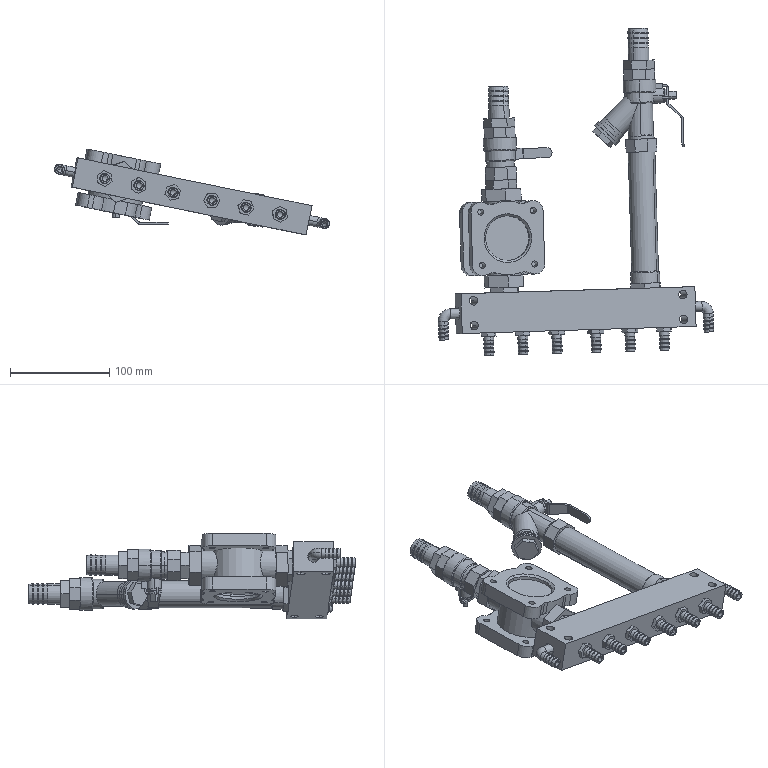Part | SolidWorks | features CompositeCurve 2 | 25 solids | 1016 faces | box 276.863 x 329.153 x 86.261 mm | volume 574652 mm3 | cylinder 419 | plane 412 | cone 162 | torus 20 | spline 3 | commonest cylinder face diameters 10 x86 20 x64 6 x26 26.1 x18 6.2 x16 11.8 x16